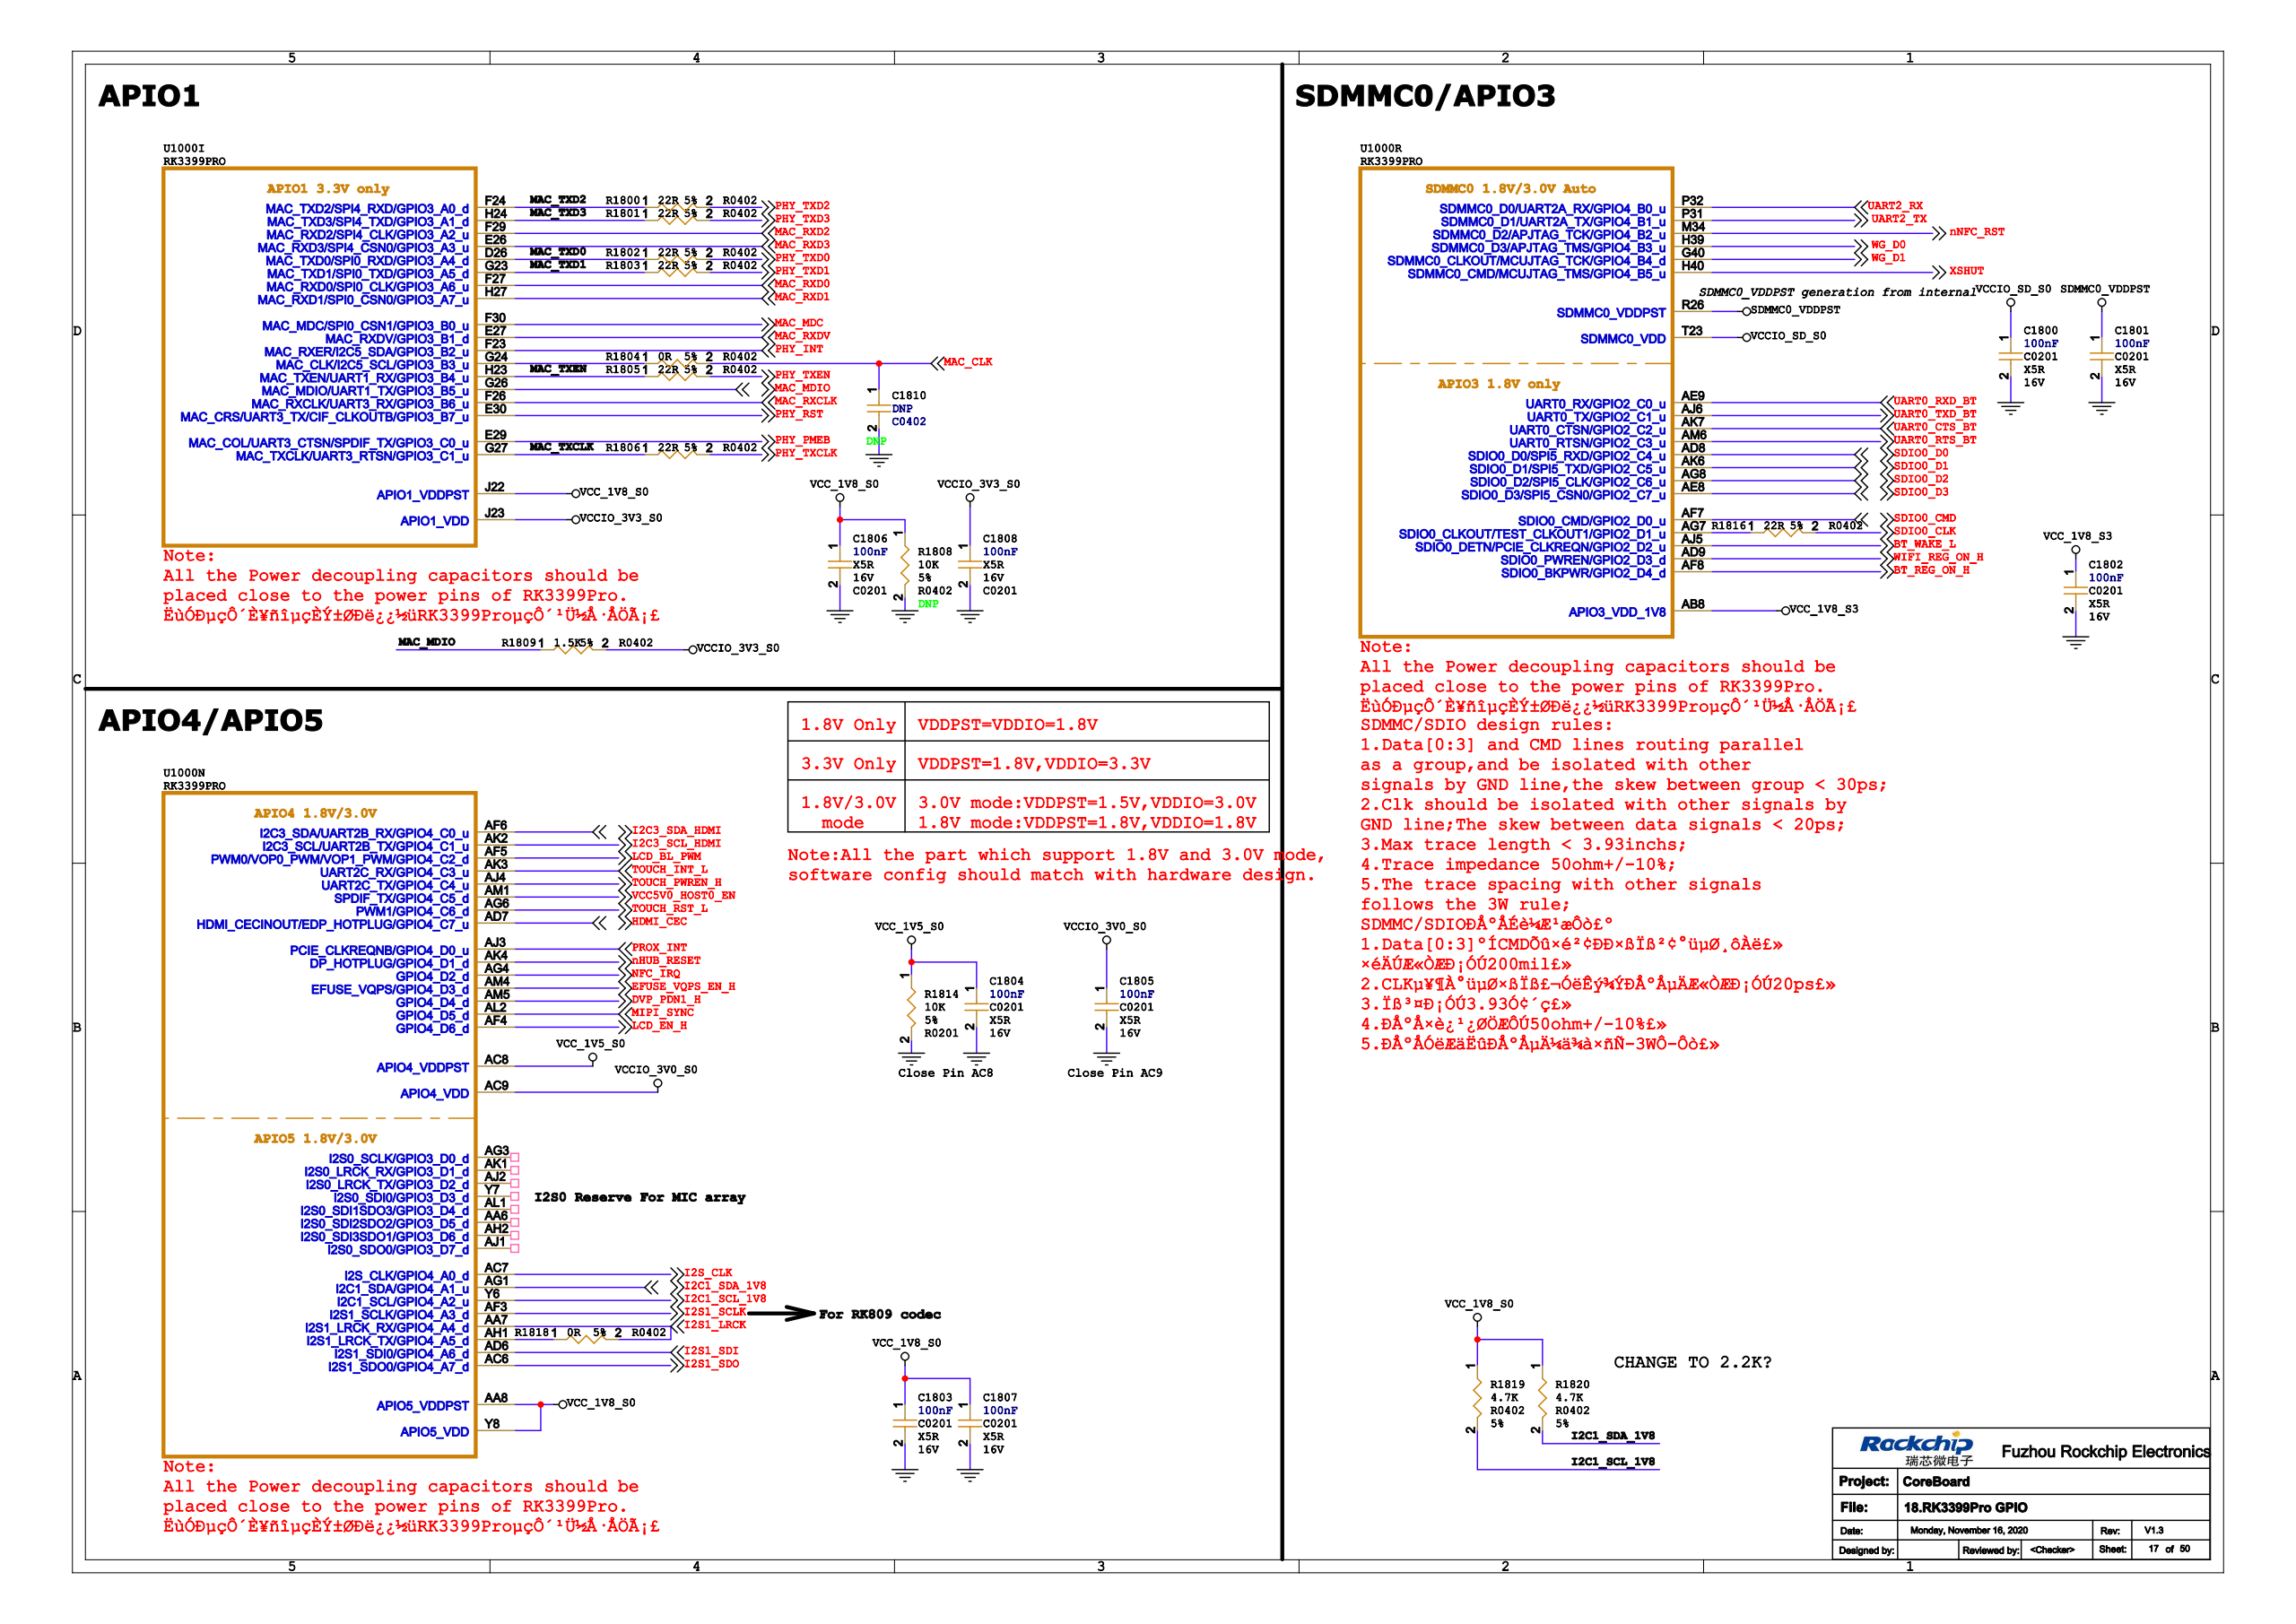Circuit board | Cadence Allegro | 749 parts | 717 nets | one sheet of the schematic
Parts on this sheet (reference | value | footprint):
C1800 | 100nF | C0201
C1801 | 100nF | C0201
C1802 | 100nF | C0201
C1803 | 100nF | C0201
C1804 | 100nF | C0201
C1805 | 100nF | C0201
C1806 | 100nF | C0201
C1807 | 100nF | C0201
C1808 | 100nF | C0201
C1810 | DNP | C0402
R1808 | 10K | R0402
R1814 | 10K | R0201
R1819 | 4.7K | R0402
R1820 | 4.7K | R0402
U1000 | RK3399PRO | BGA1372_27R00X27R00X2R19
Nets of these parts (net: part-pin ...):
GND: C1800-2 C1801-2 C1802-2 C1803-2 C1804-2 C1805-2 C1806-2 C1807-2 C1808-2 C1810-2 R1808-2 R1814-2
PHY_RST: U1000-E30
HDMI_CEC: U1000-AD7
VCC5V0_HOST0_EN: U1000-AM1
DVP_PDN1_H: U1000-AM5
TOUCH_PWREN_H: U1000-AJ4
TOUCH_INT_L: U1000-AK3
TOUCH_RST_L: U1000-AG6
VCC_1V8_S0: C1803-1 C1806-1 C1807-1 R1808-1 R1819-1 R1820-1 U1000-AA8 U1000-J22 U1000-Y8
I2C1_SDA_1V8: R1820-2 U1000-AG1
XSHUT: U1000-H40
I2C1_SCL_1V8: R1819-2 U1000-Y6
SDIO0_D0: U1000-AD8
SDIO0_D1: U1000-AK6
SDIO0_D2: U1000-AG8
SDIO0_D3: U1000-AE8
SDIO0_CMD: U1000-AF7
WG_D0: U1000-H39
WG_D1: U1000-G40
PROX_INT: U1000-AJ3
BT_WAKE_L: U1000-AJ5
BT_REG_ON_H: U1000-AF8
LCD_EN_H: U1000-AF4
LCD_BL_PWM: U1000-AF5
UART2_TX: U1000-P31
UART0_RXD_BT: U1000-AE9
UART2_RX: U1000-P32
UART0_TXD_BT: U1000-AJ6
UART0_CTS_BT: U1000-AK7
UART0_RTS_BT: U1000-AM6
WIFI_REG_ON_H: U1000-AD9
MIPI_SYNC: U1000-AL2
NFC_IRQ: U1000-AG4
VCCIO_3V3_S0: C1808-1 U1000-J23
MAC_CLK: C1810-1
PHY_INT: U1000-F23
MAC_MDC: U1000-F30
MAC_MDIO: U1000-G26
PHY_PMEB: U1000-E29
VCCIO_3V0_S0: C1805-1 U1000-AC9
I2C3_SCL_HDMI: U1000-AK2
I2C3_SDA_HDMI: U1000-AF6
VCC_1V8_S3: C1802-1 U1000-AB8
MAC_RXCLK: U1000-F26
MAC_RXD0: U1000-F27
MAC_RXD1: U1000-H27
MAC_RXD2: U1000-F29
MAC_RXD3: U1000-E26
MAC_RXDV: U1000-E27
MAC_TXCLK: U1000-G27
MAC_TXD0: U1000-D26
MAC_TXD1: U1000-G23
MAC_TXD2: U1000-F24
MAC_TXD3: U1000-H24
MAC_TXEN: U1000-H23
VCC_1V5_S0: C1804-1 R1814-1 U1000-AC8
EFUSE_VQPS_EN_H: U1000-AM4
I2S1_LRCK: U1000-AA7
I2S1_SCLK: U1000-AF3
I2S1_SDI: U1000-AD6
I2S1_SDO: U1000-AC6
I2S_CLK: U1000-AC7
VCCIO_SD_S0: C1800-1 U1000-T23
SDMMC0_VDDPST: C1801-1 U1000-R26